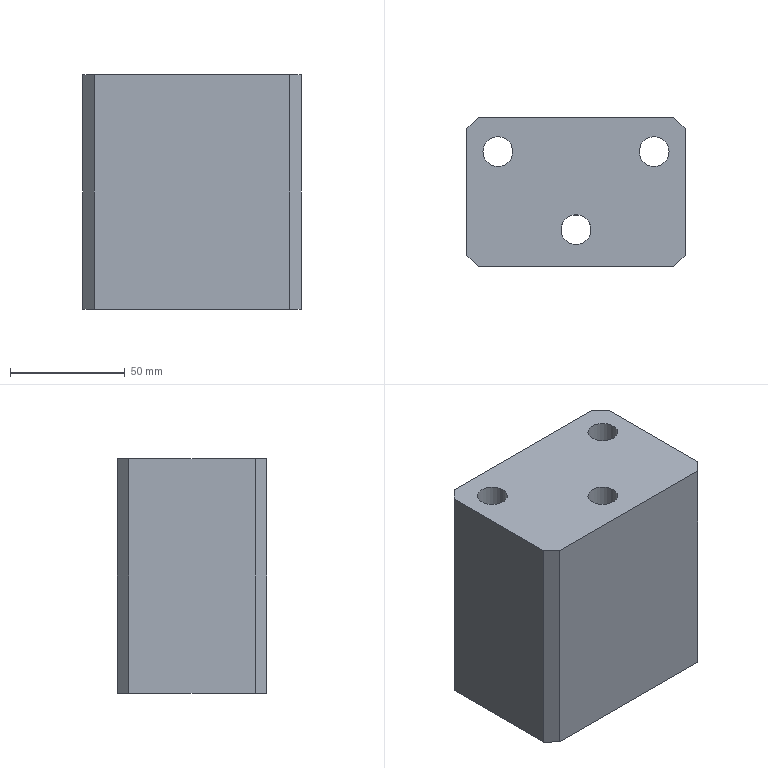Part | STEP file | gslz 2016.10.28-10_id2158_x_t | 1 solid | 28 faces | box 95 x 65 x 102 mm | volume 541267 mm3 | plane 13 | cylinder 9 | cone 6 | commonest cylinder face diameters 10.3 x3 13 x3 20 x3